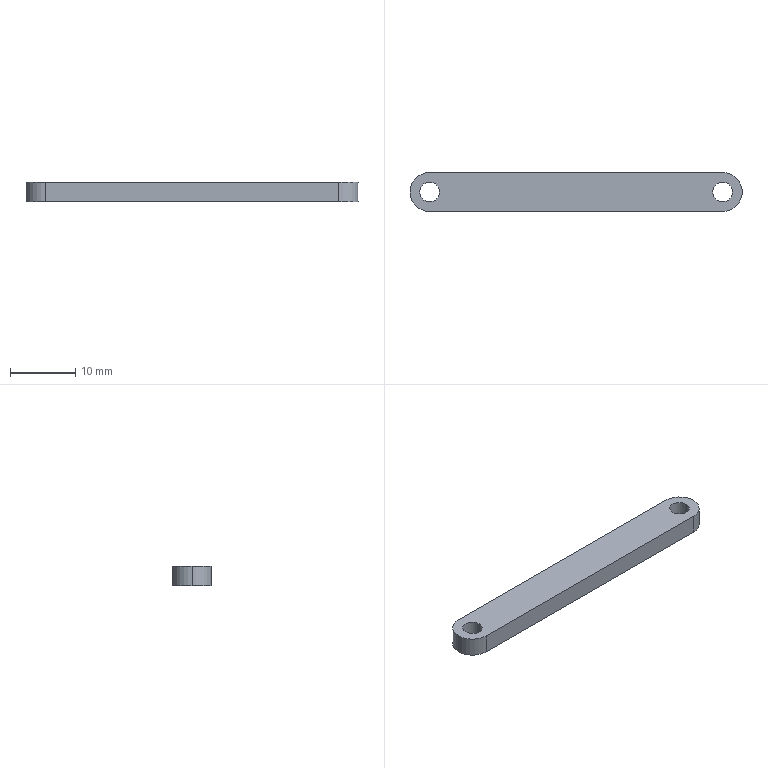Part | SolidWorks | features Extrusion 1 | 1 solid | 11 faces | box 51 x 6 x 3 mm | volume 852.412 mm3 | cylinder 7 | plane 4 | commonest cylinder face diameters 3 x4 6 x3
STEP:
#1=CARTESIAN_POINT('',(43.5,0.,3.));
#2=VERTEX_POINT('',#1);
#3=CARTESIAN_POINT('',(46.5,0.,3.));
#4=VERTEX_POINT('',#3);
#5=CARTESIAN_POINT('',(45.,0.,3.));
#6=DIRECTION('',(0.,0.,1.));
#7=DIRECTION('',(1.,0.,0.));
#8=AXIS2_PLACEMENT_3D('',#5,#6,#7);
#9=CIRCLE('',#8,1.5);
#10=EDGE_CURVE('',#2,#4,#9,.T.);
#11=ORIENTED_EDGE('',*,*,#10,.T.);
#12=CARTESIAN_POINT('',(46.5,0.,0.));
#13=VERTEX_POINT('',#12);
#14=CARTESIAN_POINT('',(46.5,0.,3.));
#15=DIRECTION('',(0.,0.,-1.));
#16=VECTOR('',#15,1000.);
#17=LINE('',#14,#16);
#18=EDGE_CURVE('',#4,#13,#17,.T.);
#19=ORIENTED_EDGE('',*,*,#18,.T.);
#20=CARTESIAN_POINT('',(43.5,0.,0.));
#21=VERTEX_POINT('',#20);
#22=CARTESIAN_POINT('',(45.,0.,0.));
#23=DIRECTION('',(0.,0.,1.));
#24=DIRECTION('',(1.,0.,0.));
#25=AXIS2_PLACEMENT_3D('',#22,#23,#24);
#26=CIRCLE('',#25,1.5);
#27=EDGE_CURVE('',#21,#13,#26,.T.);
#28=ORIENTED_EDGE('',*,*,#27,.F.);
#29=CARTESIAN_POINT('',(43.5,0.,3.));
#30=DIRECTION('',(0.,0.,-1.));
#31=VECTOR('',#30,1000.);
#32=LINE('',#29,#31);
#33=EDGE_CURVE('',#2,#21,#32,.T.);
#34=ORIENTED_EDGE('',*,*,#33,.F.);
#35=EDGE_LOOP('',(#11,#19,#28,#34));
#36=FACE_OUTER_BOUND('',#35,.T.);
#37=CARTESIAN_POINT('',(45.,0.,3.));
#38=DIRECTION('',(0.,0.,-1.));
#39=DIRECTION('',(-1.,0.,0.));
#40=AXIS2_PLACEMENT_3D('',#37,#38,#39);
#41=CYLINDRICAL_SURFACE('',#40,1.5);
#42=ADVANCED_FACE('',(#36),#41,.F.);
#43=CARTESIAN_POINT('',(-1.5,0.,3.));
#44=VERTEX_POINT('',#43);
#45=CARTESIAN_POINT('',(1.5,0.,3.));
#46=VERTEX_POINT('',#45);
#47=CARTESIAN_POINT('',(0.,0.,3.));
#48=DIRECTION('',(0.,0.,1.));
#49=DIRECTION('',(1.,0.,0.));
#50=AXIS2_PLACEMENT_3D('',#47,#48,#49);
#51=CIRCLE('',#50,1.5);
#52=EDGE_CURVE('',#44,#46,#51,.T.);
#53=ORIENTED_EDGE('',*,*,#52,.T.);
#54=CARTESIAN_POINT('',(1.5,0.,0.));
#55=VERTEX_POINT('',#54);
#56=CARTESIAN_POINT('',(1.5,0.,3.));
#57=DIRECTION('',(0.,0.,-1.));
#58=VECTOR('',#57,1000.);
#59=LINE('',#56,#58);
#60=EDGE_CURVE('',#46,#55,#59,.T.);
#61=ORIENTED_EDGE('',*,*,#60,.T.);
#62=CARTESIAN_POINT('',(-1.5,0.,0.));
#63=VERTEX_POINT('',#62);
#64=CARTESIAN_POINT('',(0.,0.,0.));
#65=DIRECTION('',(0.,0.,1.));
#66=DIRECTION('',(1.,0.,0.));
#67=AXIS2_PLACEMENT_3D('',#64,#65,#66);
#68=CIRCLE('',#67,1.5);
#69=EDGE_CURVE('',#63,#55,#68,.T.);
#70=ORIENTED_EDGE('',*,*,#69,.F.);
#71=CARTESIAN_POINT('',(-1.5,0.,3.));
#72=DIRECTION('',(0.,0.,-1.));
#73=VECTOR('',#72,1000.);
#74=LINE('',#71,#73);
#75=EDGE_CURVE('',#44,#63,#74,.T.);
#76=ORIENTED_EDGE('',*,*,#75,.F.);
#77=EDGE_LOOP('',(#53,#61,#70,#76));
#78=FACE_OUTER_BOUND('',#77,.T.);
#79=CARTESIAN_POINT('',(0.,0.,3.));
#80=DIRECTION('',(0.,0.,-1.));
#81=DIRECTION('',(-1.,0.,0.));
#82=AXIS2_PLACEMENT_3D('',#79,#80,#81);
#83=CYLINDRICAL_SURFACE('',#82,1.5);
#84=ADVANCED_FACE('',(#78),#83,.F.);
#85=CARTESIAN_POINT('',(-3.,0.,3.));
#86=VERTEX_POINT('',#85);
#87=CARTESIAN_POINT('',(0.,-3.,3.));
#88=VERTEX_POINT('',#87);
#89=CARTESIAN_POINT('',(0.,0.,3.));
#90=DIRECTION('',(0.,0.,1.));
#91=DIRECTION('',(1.,0.,0.));
#92=AXIS2_PLACEMENT_3D('',#89,#90,#91);
#93=CIRCLE('',#92,3.);
#94=EDGE_CURVE('',#86,#88,#93,.T.);
#95=ORIENTED_EDGE('',*,*,#94,.F.);
#96=CARTESIAN_POINT('',(-3.,0.,0.));
#97=VERTEX_POINT('',#96);
#98=CARTESIAN_POINT('',(-3.,0.,3.));
#99=DIRECTION('',(0.,0.,-1.));
#100=VECTOR('',#99,1000.);
#101=LINE('',#98,#100);
#102=EDGE_CURVE('',#86,#97,#101,.T.);
#103=ORIENTED_EDGE('',*,*,#102,.T.);
#104=CARTESIAN_POINT('',(0.,-3.,0.));
#105=VERTEX_POINT('',#104);
#106=CARTESIAN_POINT('',(0.,0.,0.));
#107=DIRECTION('',(0.,0.,1.));
#108=DIRECTION('',(1.,0.,0.));
#109=AXIS2_PLACEMENT_3D('',#106,#107,#108);
#110=CIRCLE('',#109,3.);
#111=EDGE_CURVE('',#97,#105,#110,.T.);
#112=ORIENTED_EDGE('',*,*,#111,.T.);
#113=CARTESIAN_POINT('',(0.,-3.,3.));
#114=DIRECTION('',(0.,0.,-1.));
#115=VECTOR('',#114,1000.);
#116=LINE('',#113,#115);
#117=EDGE_CURVE('',#88,#105,#116,.T.);
#118=ORIENTED_EDGE('',*,*,#117,.F.);
#119=EDGE_LOOP('',(#95,#103,#112,#118));
#120=FACE_OUTER_BOUND('',#119,.T.);
#121=CARTESIAN_POINT('',(0.,0.,3.));
#122=DIRECTION('',(0.,0.,-1.));
#123=DIRECTION('',(-1.,0.,0.));
#124=AXIS2_PLACEMENT_3D('',#121,#122,#123);
#125=CYLINDRICAL_SURFACE('',#124,3.);
#126=ADVANCED_FACE('',(#120),#125,.T.);
#127=ORIENTED_EDGE('',*,*,#52,.F.);
#128=CARTESIAN_POINT('',(0.,0.,3.));
#129=DIRECTION('',(0.,0.,1.));
#130=DIRECTION('',(1.,0.,0.));
#131=AXIS2_PLACEMENT_3D('',#128,#129,#130);
#132=CIRCLE('',#131,1.5);
#133=EDGE_CURVE('',#46,#44,#132,.T.);
#134=ORIENTED_EDGE('',*,*,#133,.F.);
#135=EDGE_LOOP('',(#127,#134));
#136=FACE_BOUND('',#135,.T.);
#137=CARTESIAN_POINT('',(0.,3.,3.));
#138=VERTEX_POINT('',#137);
#139=CARTESIAN_POINT('',(0.,0.,3.));
#140=DIRECTION('',(0.,0.,1.));
#141=DIRECTION('',(1.,0.,0.));
#142=AXIS2_PLACEMENT_3D('',#139,#140,#141);
#143=CIRCLE('',#142,3.);
#144=EDGE_CURVE('',#138,#86,#143,.T.);
#145=ORIENTED_EDGE('',*,*,#144,.T.);
#146=ORIENTED_EDGE('',*,*,#94,.T.);
#147=CARTESIAN_POINT('',(45.,-3.,3.));
#148=VERTEX_POINT('',#147);
#149=CARTESIAN_POINT('',(0.,-3.,3.));
#150=DIRECTION('',(1.,0.,0.));
#151=VECTOR('',#150,1000.);
#152=LINE('',#149,#151);
#153=EDGE_CURVE('',#88,#148,#152,.T.);
#154=ORIENTED_EDGE('',*,*,#153,.T.);
#155=CARTESIAN_POINT('',(45.,3.,3.));
#156=VERTEX_POINT('',#155);
#157=CARTESIAN_POINT('',(45.,0.,3.));
#158=DIRECTION('',(0.,0.,1.));
#159=DIRECTION('',(1.,0.,0.));
#160=AXIS2_PLACEMENT_3D('',#157,#158,#159);
#161=CIRCLE('',#160,3.);
#162=EDGE_CURVE('',#148,#156,#161,.T.);
#163=ORIENTED_EDGE('',*,*,#162,.T.);
#164=CARTESIAN_POINT('',(0.,3.,3.));
#165=DIRECTION('',(-1.,0.,0.));
#166=VECTOR('',#165,1000.);
#167=LINE('',#164,#166);
#168=EDGE_CURVE('',#156,#138,#167,.T.);
#169=ORIENTED_EDGE('',*,*,#168,.T.);
#170=EDGE_LOOP('',(#145,#146,#154,#163,#169));
#171=FACE_OUTER_BOUND('',#170,.T.);
#172=ORIENTED_EDGE('',*,*,#10,.F.);
#173=CARTESIAN_POINT('',(45.,0.,3.));
#174=DIRECTION('',(0.,0.,1.));
#175=DIRECTION('',(1.,0.,0.));
#176=AXIS2_PLACEMENT_3D('',#173,#174,#175);
#177=CIRCLE('',#176,1.5);
#178=EDGE_CURVE('',#4,#2,#177,.T.);
#179=ORIENTED_EDGE('',*,*,#178,.F.);
#180=EDGE_LOOP('',(#172,#179));
#181=FACE_BOUND('',#180,.T.);
#182=CARTESIAN_POINT('',(0.,0.,3.));
#183=DIRECTION('',(0.,0.,1.));
#184=DIRECTION('',(1.,0.,0.));
#185=AXIS2_PLACEMENT_3D('',#182,#183,#184);
#186=PLANE('',#185);
#187=ADVANCED_FACE('',(#136,#171,#181),#186,.T.);
#188=CARTESIAN_POINT('',(0.,3.,0.));
#189=VERTEX_POINT('',#188);
#190=CARTESIAN_POINT('',(0.,0.,0.));
#191=DIRECTION('',(0.,0.,1.));
#192=DIRECTION('',(1.,0.,0.));
#193=AXIS2_PLACEMENT_3D('',#190,#191,#192);
#194=CIRCLE('',#193,3.);
#195=EDGE_CURVE('',#189,#97,#194,.T.);
#196=ORIENTED_EDGE('',*,*,#195,.F.);
#197=CARTESIAN_POINT('',(45.,3.,0.));
#198=VERTEX_POINT('',#197);
#199=CARTESIAN_POINT('',(0.,3.,0.));
#200=DIRECTION('',(-1.,0.,0.));
#201=VECTOR('',#200,1000.);
#202=LINE('',#199,#201);
#203=EDGE_CURVE('',#198,#189,#202,.T.);
#204=ORIENTED_EDGE('',*,*,#203,.F.);
#205=CARTESIAN_POINT('',(45.,-3.,0.));
#206=VERTEX_POINT('',#205);
#207=CARTESIAN_POINT('',(45.,0.,0.));
#208=DIRECTION('',(0.,0.,1.));
#209=DIRECTION('',(1.,0.,0.));
#210=AXIS2_PLACEMENT_3D('',#207,#208,#209);
#211=CIRCLE('',#210,3.);
#212=EDGE_CURVE('',#206,#198,#211,.T.);
#213=ORIENTED_EDGE('',*,*,#212,.F.);
#214=CARTESIAN_POINT('',(0.,-3.,0.));
#215=DIRECTION('',(1.,0.,0.));
#216=VECTOR('',#215,1000.);
#217=LINE('',#214,#216);
#218=EDGE_CURVE('',#105,#206,#217,.T.);
#219=ORIENTED_EDGE('',*,*,#218,.F.);
#220=ORIENTED_EDGE('',*,*,#111,.F.);
#221=EDGE_LOOP('',(#196,#204,#213,#219,#220));
#222=FACE_OUTER_BOUND('',#221,.T.);
#223=ORIENTED_EDGE('',*,*,#69,.T.);
#224=CARTESIAN_POINT('',(0.,0.,0.));
#225=DIRECTION('',(0.,0.,1.));
#226=DIRECTION('',(1.,0.,0.));
#227=AXIS2_PLACEMENT_3D('',#224,#225,#226);
#228=CIRCLE('',#227,1.5);
#229=EDGE_CURVE('',#55,#63,#228,.T.);
#230=ORIENTED_EDGE('',*,*,#229,.T.);
#231=EDGE_LOOP('',(#223,#230));
#232=FACE_BOUND('',#231,.T.);
#233=ORIENTED_EDGE('',*,*,#27,.T.);
#234=CARTESIAN_POINT('',(45.,0.,0.));
#235=DIRECTION('',(0.,0.,1.));
#236=DIRECTION('',(1.,0.,0.));
#237=AXIS2_PLACEMENT_3D('',#234,#235,#236);
#238=CIRCLE('',#237,1.5);
#239=EDGE_CURVE('',#13,#21,#238,.T.);
#240=ORIENTED_EDGE('',*,*,#239,.T.);
#241=EDGE_LOOP('',(#233,#240));
#242=FACE_BOUND('',#241,.T.);
#243=CARTESIAN_POINT('',(0.,0.,0.));
#244=DIRECTION('',(0.,0.,1.));
#245=DIRECTION('',(1.,0.,0.));
#246=AXIS2_PLACEMENT_3D('',#243,#244,#245);
#247=PLANE('',#246);
#248=ADVANCED_FACE('',(#222,#232,#242),#247,.F.);
#249=ORIENTED_EDGE('',*,*,#102,.F.);
#250=ORIENTED_EDGE('',*,*,#144,.F.);
#251=CARTESIAN_POINT('',(0.,3.,3.));
#252=DIRECTION('',(0.,0.,-1.));
#253=VECTOR('',#252,1000.);
#254=LINE('',#251,#253);
#255=EDGE_CURVE('',#138,#189,#254,.T.);
#256=ORIENTED_EDGE('',*,*,#255,.T.);
#257=ORIENTED_EDGE('',*,*,#195,.T.);
#258=EDGE_LOOP('',(#249,#250,#256,#257));
#259=FACE_OUTER_BOUND('',#258,.T.);
#260=CARTESIAN_POINT('',(0.,0.,3.));
#261=DIRECTION('',(0.,0.,-1.));
#262=DIRECTION('',(-1.,0.,0.));
#263=AXIS2_PLACEMENT_3D('',#260,#261,#262);
#264=CYLINDRICAL_SURFACE('',#263,3.);
#265=ADVANCED_FACE('',(#259),#264,.T.);
#266=ORIENTED_EDGE('',*,*,#218,.T.);
#267=CARTESIAN_POINT('',(45.,-3.,3.));
#268=DIRECTION('',(0.,0.,-1.));
#269=VECTOR('',#268,1000.);
#270=LINE('',#267,#269);
#271=EDGE_CURVE('',#148,#206,#270,.T.);
#272=ORIENTED_EDGE('',*,*,#271,.F.);
#273=ORIENTED_EDGE('',*,*,#153,.F.);
#274=ORIENTED_EDGE('',*,*,#117,.T.);
#275=EDGE_LOOP('',(#266,#272,#273,#274));
#276=FACE_OUTER_BOUND('',#275,.T.);
#277=CARTESIAN_POINT('',(0.,-3.,3.));
#278=DIRECTION('',(0.,1.,0.));
#279=DIRECTION('',(-1.,0.,0.));
#280=AXIS2_PLACEMENT_3D('',#277,#278,#279);
#281=PLANE('',#280);
#282=ADVANCED_FACE('',(#276),#281,.F.);
#283=ORIENTED_EDGE('',*,*,#212,.T.);
#284=CARTESIAN_POINT('',(45.,3.,3.));
#285=DIRECTION('',(0.,0.,-1.));
#286=VECTOR('',#285,1000.);
#287=LINE('',#284,#286);
#288=EDGE_CURVE('',#156,#198,#287,.T.);
#289=ORIENTED_EDGE('',*,*,#288,.F.);
#290=ORIENTED_EDGE('',*,*,#162,.F.);
#291=ORIENTED_EDGE('',*,*,#271,.T.);
#292=EDGE_LOOP('',(#283,#289,#290,#291));
#293=FACE_OUTER_BOUND('',#292,.T.);
#294=CARTESIAN_POINT('',(45.,0.,3.));
#295=DIRECTION('',(0.,0.,-1.));
#296=DIRECTION('',(-1.,0.,0.));
#297=AXIS2_PLACEMENT_3D('',#294,#295,#296);
#298=CYLINDRICAL_SURFACE('',#297,3.);
#299=ADVANCED_FACE('',(#293),#298,.T.);
#300=ORIENTED_EDGE('',*,*,#203,.T.);
#301=ORIENTED_EDGE('',*,*,#255,.F.);
#302=ORIENTED_EDGE('',*,*,#168,.F.);
#303=ORIENTED_EDGE('',*,*,#288,.T.);
#304=EDGE_LOOP('',(#300,#301,#302,#303));
#305=FACE_OUTER_BOUND('',#304,.T.);
#306=CARTESIAN_POINT('',(0.,3.,3.));
#307=DIRECTION('',(0.,-1.,0.));
#308=DIRECTION('',(1.,0.,0.));
#309=AXIS2_PLACEMENT_3D('',#306,#307,#308);
#310=PLANE('',#309);
#311=ADVANCED_FACE('',(#305),#310,.F.);
#312=ORIENTED_EDGE('',*,*,#60,.F.);
#313=ORIENTED_EDGE('',*,*,#133,.T.);
#314=ORIENTED_EDGE('',*,*,#75,.T.);
#315=ORIENTED_EDGE('',*,*,#229,.F.);
#316=EDGE_LOOP('',(#312,#313,#314,#315));
#317=FACE_OUTER_BOUND('',#316,.T.);
#318=CARTESIAN_POINT('',(0.,0.,3.));
#319=DIRECTION('',(0.,0.,-1.));
#320=DIRECTION('',(-1.,0.,0.));
#321=AXIS2_PLACEMENT_3D('',#318,#319,#320);
#322=CYLINDRICAL_SURFACE('',#321,1.5);
#323=ADVANCED_FACE('',(#317),#322,.F.);
#324=ORIENTED_EDGE('',*,*,#18,.F.);
#325=ORIENTED_EDGE('',*,*,#178,.T.);
#326=ORIENTED_EDGE('',*,*,#33,.T.);
#327=ORIENTED_EDGE('',*,*,#239,.F.);
#328=EDGE_LOOP('',(#324,#325,#326,#327));
#329=FACE_OUTER_BOUND('',#328,.T.);
#330=CARTESIAN_POINT('',(45.,0.,3.));
#331=DIRECTION('',(0.,0.,-1.));
#332=DIRECTION('',(-1.,0.,0.));
#333=AXIS2_PLACEMENT_3D('',#330,#331,#332);
#334=CYLINDRICAL_SURFACE('',#333,1.5);
#335=ADVANCED_FACE('',(#329),#334,.F.);
#336=CLOSED_SHELL('',(#42,#84,#126,#187,#248,#265,#282,#299,#311,#323,#335));
#337=MANIFOLD_SOLID_BREP('',#336);
#338=CARTESIAN_POINT('',(0.,0.,0.));
#339=DIRECTION('',(0.,0.,1.));
#340=DIRECTION('',(1.,0.,0.));
#341=AXIS2_PLACEMENT_3D('',#338,#339,#340);
#342=(LENGTH_UNIT()NAMED_UNIT(*)SI_UNIT(.MILLI.,.METRE.));
#343=UNCERTAINTY_MEASURE_WITH_UNIT(LENGTH_MEASURE(0.00001),#342,'','');
#344=(NAMED_UNIT(*)PLANE_ANGLE_UNIT()SI_UNIT($,.RADIAN.));
#345=(NAMED_UNIT(*)SI_UNIT($,.STERADIAN.)SOLID_ANGLE_UNIT());
#346=(GEOMETRIC_REPRESENTATION_CONTEXT(3)GLOBAL_UNCERTAINTY_ASSIGNED_CONTEXT((#343))GLOBAL_UNIT_ASSIGNED_CONTEXT((#342,#344,#345))REPRESENTATION_CONTEXT('',''));
#347=ADVANCED_BREP_SHAPE_REPRESENTATION('',(#337,#341),#346);